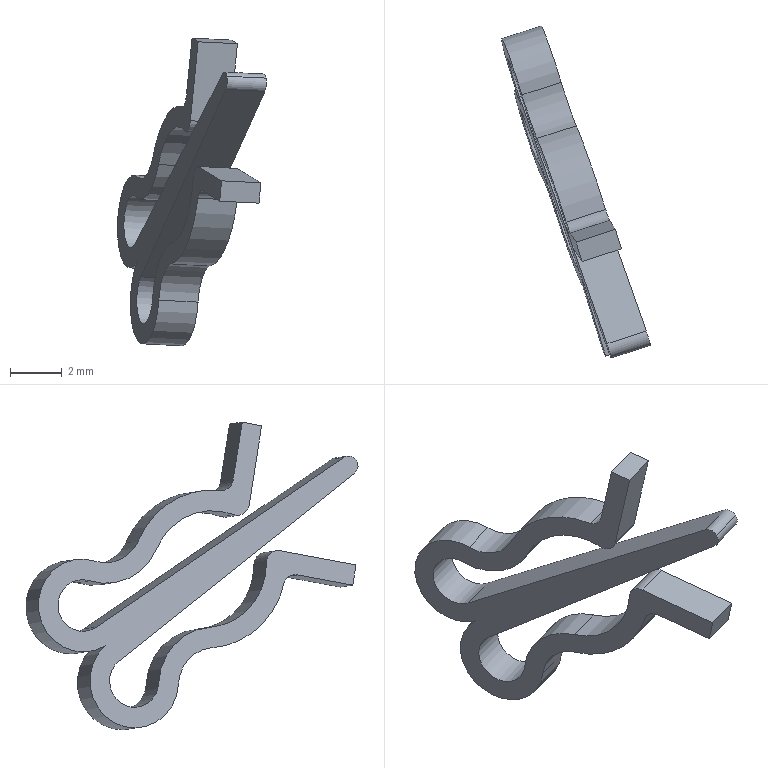Part | SolidWorks | features BaseBody 1 | 1 solid | 28 faces | box 5.768 x 12.862 x 11.907 mm | volume 63.823 mm3 | cylinder 18 | plane 10 | commonest cylinder face diameters 0.745 x2 0.982 x2 1 x2 2 x2 3 x2 3.6 x2
STEP:
#1=CARTESIAN_POINT('',(66.487,-82.448,-179.895));
#2=VERTEX_POINT('',#1);
#3=CARTESIAN_POINT('',(66.439,-82.377,-180.405));
#4=VERTEX_POINT('',#3);
#5=CARTESIAN_POINT('',(66.384,-82.16,-180.108));
#6=DIRECTION('',(0.9511,0.3055,-0.04654));
#7=DIRECTION('',(-0.2762,0.7728,-0.5713));
#8=AXIS2_PLACEMENT_3D('',#5,#6,#7);
#9=CIRCLE('',#8,0.3723);
#10=EDGE_CURVE('',#2,#4,#9,.T.);
#11=ORIENTED_EDGE('',*,*,#10,.F.);
#12=CARTESIAN_POINT('',(64.965,-82.936,-179.82));
#13=VERTEX_POINT('',#12);
#14=CARTESIAN_POINT('',(66.487,-82.448,-179.895));
#15=DIRECTION('',(-0.9511,-0.3055,0.04654));
#16=VECTOR('',#15,1000.);
#17=LINE('',#14,#16);
#18=EDGE_CURVE('',#2,#13,#17,.T.);
#19=ORIENTED_EDGE('',*,*,#18,.T.);
#20=CARTESIAN_POINT('',(64.918,-82.866,-180.331));
#21=VERTEX_POINT('',#20);
#22=CARTESIAN_POINT('',(64.863,-82.649,-180.033));
#23=DIRECTION('',(0.9511,0.3055,-0.04654));
#24=DIRECTION('',(-0.2762,0.7728,-0.5713));
#25=AXIS2_PLACEMENT_3D('',#22,#23,#24);
#26=CIRCLE('',#25,0.3723);
#27=EDGE_CURVE('',#13,#21,#26,.T.);
#28=ORIENTED_EDGE('',*,*,#27,.T.);
#29=CARTESIAN_POINT('',(66.439,-82.377,-180.405));
#30=DIRECTION('',(-0.9511,-0.3055,0.04654));
#31=VECTOR('',#30,1000.);
#32=LINE('',#29,#31);
#33=EDGE_CURVE('',#4,#21,#32,.T.);
#34=ORIENTED_EDGE('',*,*,#33,.F.);
#35=EDGE_LOOP('',(#11,#19,#28,#34));
#36=FACE_OUTER_BOUND('',#35,.T.);
#37=CARTESIAN_POINT('',(66.384,-82.16,-180.108));
#38=DIRECTION('',(-0.9511,-0.3055,0.04654));
#39=DIRECTION('',(0.2762,-0.7728,0.5713));
#40=AXIS2_PLACEMENT_3D('',#37,#38,#39);
#41=CYLINDRICAL_SURFACE('',#40,0.3723);
#42=ADVANCED_FACE('',(#36),#41,.T.);
#43=CARTESIAN_POINT('',(64.815,-82.452,-179.721));
#44=VERTEX_POINT('',#43);
#45=CARTESIAN_POINT('',(64.863,-82.649,-180.033));
#46=DIRECTION('',(0.9511,0.3055,-0.04654));
#47=DIRECTION('',(-0.2762,0.7728,-0.5713));
#48=AXIS2_PLACEMENT_3D('',#45,#46,#47);
#49=CIRCLE('',#48,0.3723);
#50=EDGE_CURVE('',#44,#13,#49,.T.);
#51=ORIENTED_EDGE('',*,*,#50,.F.);
#52=CARTESIAN_POINT('',(61.417,-72.873,-186.282));
#53=VERTEX_POINT('',#52);
#54=CARTESIAN_POINT('',(64.815,-82.452,-179.721));
#55=DIRECTION('',(0.2809,-0.7918,0.5424));
#56=VECTOR('',#55,1000.);
#57=LINE('',#54,#56);
#58=EDGE_CURVE('',#53,#44,#57,.T.);
#59=ORIENTED_EDGE('',*,*,#58,.F.);
#60=CARTESIAN_POINT('',(61.419,-72.607,-184.488));
#61=VERTEX_POINT('',#60);
#62=CARTESIAN_POINT('',(61.288,-72.344,-185.444));
#63=DIRECTION('',(-0.9511,-0.3055,0.04654));
#64=DIRECTION('',(-0.2762,0.7728,-0.5713));
#65=AXIS2_PLACEMENT_3D('',#62,#63,#64);
#66=CIRCLE('',#65,1.);
#67=EDGE_CURVE('',#61,#53,#66,.T.);
#68=ORIENTED_EDGE('',*,*,#67,.F.);
#69=CARTESIAN_POINT('',(62.319,-75.217,-183.241));
#70=VERTEX_POINT('',#69);
#71=CARTESIAN_POINT('',(61.721,-73.211,-182.289));
#72=DIRECTION('',(0.9511,0.3055,-0.04654));
#73=DIRECTION('',(-0.2762,0.7728,-0.5713));
#74=AXIS2_PLACEMENT_3D('',#71,#72,#73);
#75=CIRCLE('',#74,2.3);
#76=EDGE_CURVE('',#70,#61,#75,.T.);
#77=ORIENTED_EDGE('',*,*,#76,.F.);
#78=CARTESIAN_POINT('',(63.335,-78.182,-181.921));
#79=VERTEX_POINT('',#78);
#80=CARTESIAN_POINT('',(62.971,-77.406,-184.279));
#81=DIRECTION('',(-0.9511,-0.3055,0.04654));
#82=DIRECTION('',(-0.2762,0.7728,-0.5713));
#83=AXIS2_PLACEMENT_3D('',#80,#81,#82);
#84=CIRCLE('',#83,2.509);
#85=EDGE_CURVE('',#79,#70,#84,.T.);
#86=ORIENTED_EDGE('',*,*,#85,.F.);
#87=CARTESIAN_POINT('',(63.551,-78.795,-181.546));
#88=VERTEX_POINT('',#87);
#89=CARTESIAN_POINT('',(63.407,-78.334,-181.46));
#90=DIRECTION('',(0.9511,0.3055,-0.04654));
#91=DIRECTION('',(0.2762,-0.7728,0.5713));
#92=AXIS2_PLACEMENT_3D('',#89,#90,#91);
#93=CIRCLE('',#92,0.491);
#94=EDGE_CURVE('',#88,#79,#93,.T.);
#95=ORIENTED_EDGE('',*,*,#94,.F.);
#96=CARTESIAN_POINT('',(63.853,-79.272,-178.489));
#97=VERTEX_POINT('',#96);
#98=CARTESIAN_POINT('',(63.853,-79.272,-178.489));
#99=DIRECTION('',(-0.09732,0.1532,-0.9834));
#100=VECTOR('',#99,1000.);
#101=LINE('',#98,#100);
#102=EDGE_CURVE('',#97,#88,#101,.T.);
#103=ORIENTED_EDGE('',*,*,#102,.F.);
#104=CARTESIAN_POINT('',(63.619,-78.52,-178.348));
#105=VERTEX_POINT('',#104);
#106=CARTESIAN_POINT('',(63.853,-79.272,-178.489));
#107=DIRECTION('',(0.2933,-0.9398,-0.1754));
#108=VECTOR('',#107,1000.);
#109=LINE('',#106,#108);
#110=EDGE_CURVE('',#105,#97,#109,.T.);
#111=ORIENTED_EDGE('',*,*,#110,.F.);
#112=CARTESIAN_POINT('',(63.397,-78.171,-180.587));
#113=VERTEX_POINT('',#112);
#114=CARTESIAN_POINT('',(63.619,-78.52,-178.348));
#115=DIRECTION('',(0.09732,-0.1532,0.9834));
#116=VECTOR('',#115,1000.);
#117=LINE('',#114,#116);
#118=EDGE_CURVE('',#113,#105,#117,.T.);
#119=ORIENTED_EDGE('',*,*,#118,.F.);
#120=CARTESIAN_POINT('',(63.24,-77.743,-180.997));
#121=VERTEX_POINT('',#120);
#122=CARTESIAN_POINT('',(63.251,-77.701,-180.499));
#123=DIRECTION('',(-0.9511,-0.3055,0.04654));
#124=DIRECTION('',(-0.2762,0.7728,-0.5713));
#125=AXIS2_PLACEMENT_3D('',#122,#123,#124);
#126=CIRCLE('',#125,0.5);
#127=EDGE_CURVE('',#121,#113,#126,.T.);
#128=ORIENTED_EDGE('',*,*,#127,.F.);
#129=CARTESIAN_POINT('',(62.103,-74.502,-182.95));
#130=VERTEX_POINT('',#129);
#131=CARTESIAN_POINT('',(62.971,-77.406,-184.279));
#132=DIRECTION('',(0.9511,0.3055,-0.04654));
#133=DIRECTION('',(-0.2762,0.7728,-0.5713));
#134=AXIS2_PLACEMENT_3D('',#131,#132,#133);
#135=CIRCLE('',#134,3.31);
#136=EDGE_CURVE('',#130,#121,#135,.T.);
#137=ORIENTED_EDGE('',*,*,#136,.F.);
#138=CARTESIAN_POINT('',(61.524,-72.817,-183.723));
#139=VERTEX_POINT('',#138);
#140=CARTESIAN_POINT('',(61.721,-73.211,-182.289));
#141=DIRECTION('',(-0.9511,-0.3055,0.04654));
#142=DIRECTION('',(-0.2762,0.7728,-0.5713));
#143=AXIS2_PLACEMENT_3D('',#140,#141,#142);
#144=CIRCLE('',#143,1.5);
#145=EDGE_CURVE('',#139,#130,#144,.T.);
#146=ORIENTED_EDGE('',*,*,#145,.F.);
#147=CARTESIAN_POINT('',(61.495,-73.225,-187.));
#148=VERTEX_POINT('',#147);
#149=CARTESIAN_POINT('',(61.288,-72.344,-185.444));
#150=DIRECTION('',(0.9511,0.3055,-0.04654));
#151=DIRECTION('',(-0.2762,0.7728,-0.5713));
#152=AXIS2_PLACEMENT_3D('',#149,#150,#151);
#153=CIRCLE('',#152,1.8);
#154=EDGE_CURVE('',#148,#139,#153,.T.);
#155=ORIENTED_EDGE('',*,*,#154,.F.);
#156=CARTESIAN_POINT('',(62.33,-76.052,-188.489));
#157=VERTEX_POINT('',#156);
#158=CARTESIAN_POINT('',(61.785,-74.339,-188.383));
#159=DIRECTION('',(0.9511,0.3055,-0.04654));
#160=DIRECTION('',(0.2762,-0.7728,0.5713));
#161=AXIS2_PLACEMENT_3D('',#158,#159,#160);
#162=CIRCLE('',#161,1.8);
#163=EDGE_CURVE('',#157,#148,#162,.T.);
#164=ORIENTED_EDGE('',*,*,#163,.F.);
#165=CARTESIAN_POINT('',(62.802,-77.309,-187.086));
#166=VERTEX_POINT('',#165);
#167=CARTESIAN_POINT('',(62.784,-77.479,-188.576));
#168=DIRECTION('',(-0.9511,-0.3055,0.04654));
#169=DIRECTION('',(0.2762,-0.7728,0.5713));
#170=AXIS2_PLACEMENT_3D('',#167,#168,#169);
#171=CIRCLE('',#170,1.5);
#172=EDGE_CURVE('',#166,#157,#171,.T.);
#173=ORIENTED_EDGE('',*,*,#172,.F.);
#174=CARTESIAN_POINT('',(63.839,-80.15,-184.543));
#175=VERTEX_POINT('',#174);
#176=CARTESIAN_POINT('',(62.887,-77.071,-183.786));
#177=DIRECTION('',(0.9511,0.3055,-0.04654));
#178=DIRECTION('',(0.2762,-0.7728,0.5713));
#179=AXIS2_PLACEMENT_3D('',#176,#177,#178);
#180=CIRCLE('',#179,3.31);
#181=EDGE_CURVE('',#175,#166,#180,.T.);
#182=ORIENTED_EDGE('',*,*,#181,.F.);
#183=CARTESIAN_POINT('',(64.018,-80.663,-184.258));
#184=VERTEX_POINT('',#183);
#185=CARTESIAN_POINT('',(63.969,-80.586,-184.749));
#186=DIRECTION('',(-0.9511,-0.3055,0.04654));
#187=DIRECTION('',(0.2762,-0.7728,0.5713));
#188=AXIS2_PLACEMENT_3D('',#185,#186,#187);
#189=CIRCLE('',#188,0.5);
#190=EDGE_CURVE('',#184,#175,#189,.T.);
#191=ORIENTED_EDGE('',*,*,#190,.F.);
#192=CARTESIAN_POINT('',(64.686,-82.802,-184.657));
#193=VERTEX_POINT('',#192);
#194=CARTESIAN_POINT('',(64.686,-82.802,-184.657));
#195=DIRECTION('',(-0.2933,0.9398,0.1754));
#196=VECTOR('',#195,1000.);
#197=LINE('',#194,#196);
#198=EDGE_CURVE('',#193,#184,#197,.T.);
#199=ORIENTED_EDGE('',*,*,#198,.F.);
#200=CARTESIAN_POINT('',(64.763,-82.925,-183.87));
#201=VERTEX_POINT('',#200);
#202=CARTESIAN_POINT('',(64.763,-82.925,-183.87));
#203=DIRECTION('',(-0.09732,0.1532,-0.9834));
#204=VECTOR('',#203,1000.);
#205=LINE('',#202,#204);
#206=EDGE_CURVE('',#201,#193,#205,.T.);
#207=ORIENTED_EDGE('',*,*,#206,.F.);
#208=CARTESIAN_POINT('',(63.852,-80.003,-183.325));
#209=VERTEX_POINT('',#208);
#210=CARTESIAN_POINT('',(64.763,-82.925,-183.87));
#211=DIRECTION('',(0.2933,-0.9398,-0.1754));
#212=VECTOR('',#211,1000.);
#213=LINE('',#210,#212);
#214=EDGE_CURVE('',#209,#201,#213,.T.);
#215=ORIENTED_EDGE('',*,*,#214,.F.);
#216=CARTESIAN_POINT('',(63.654,-79.46,-183.804));
#217=VERTEX_POINT('',#216);
#218=CARTESIAN_POINT('',(63.804,-79.928,-183.808));
#219=DIRECTION('',(0.9511,0.3055,-0.04654));
#220=DIRECTION('',(-0.2762,0.7728,-0.5713));
#221=AXIS2_PLACEMENT_3D('',#218,#219,#220);
#222=CIRCLE('',#221,0.491);
#223=EDGE_CURVE('',#217,#209,#222,.T.);
#224=ORIENTED_EDGE('',*,*,#223,.F.);
#225=CARTESIAN_POINT('',(62.833,-77.284,-186.285));
#226=VERTEX_POINT('',#225);
#227=CARTESIAN_POINT('',(62.887,-77.071,-183.786));
#228=DIRECTION('',(-0.9511,-0.3055,0.04654));
#229=DIRECTION('',(0.2762,-0.7728,0.5713));
#230=AXIS2_PLACEMENT_3D('',#227,#228,#229);
#231=CIRCLE('',#230,2.509);
#232=EDGE_CURVE('',#226,#217,#231,.T.);
#233=ORIENTED_EDGE('',*,*,#232,.F.);
#234=CARTESIAN_POINT('',(62.088,-75.291,-188.442));
#235=VERTEX_POINT('',#234);
#236=CARTESIAN_POINT('',(62.784,-77.479,-188.576));
#237=DIRECTION('',(0.9511,0.3055,-0.04654));
#238=DIRECTION('',(0.2762,-0.7728,0.5713));
#239=AXIS2_PLACEMENT_3D('',#236,#237,#238);
#240=CIRCLE('',#239,2.3);
#241=EDGE_CURVE('',#235,#226,#240,.T.);
#242=ORIENTED_EDGE('',*,*,#241,.F.);
#243=CARTESIAN_POINT('',(61.637,-73.757,-187.584));
#244=VERTEX_POINT('',#243);
#245=CARTESIAN_POINT('',(61.785,-74.339,-188.383));
#246=DIRECTION('',(-0.9511,-0.3055,0.04654));
#247=DIRECTION('',(0.2762,-0.7728,0.5713));
#248=AXIS2_PLACEMENT_3D('',#245,#246,#247);
#249=CIRCLE('',#248,1.);
#250=EDGE_CURVE('',#244,#235,#249,.T.);
#251=ORIENTED_EDGE('',*,*,#250,.F.);
#252=CARTESIAN_POINT('',(64.918,-82.866,-180.331));
#253=DIRECTION('',(-0.2712,0.753,-0.5996));
#254=VECTOR('',#253,1000.);
#255=LINE('',#252,#254);
#256=EDGE_CURVE('',#21,#244,#255,.T.);
#257=ORIENTED_EDGE('',*,*,#256,.F.);
#258=ORIENTED_EDGE('',*,*,#27,.F.);
#259=EDGE_LOOP('',(#51,#59,#68,#77,#86,#95,#103,#111,#119,#128,#137,#146,#155,#164,#173,#182,#191,#199,#207,#215,#224,#233,#242,#251,#257,#258));
#260=FACE_OUTER_BOUND('',#259,.T.);
#261=CARTESIAN_POINT('',(64.863,-82.649,-180.033));
#262=DIRECTION('',(0.9511,0.3055,-0.04654));
#263=DIRECTION('',(0.,-0.1506,-0.9886));
#264=AXIS2_PLACEMENT_3D('',#261,#262,#263);
#265=PLANE('',#264);
#266=ADVANCED_FACE('',(#260),#265,.F.);
#267=CARTESIAN_POINT('',(66.336,-81.963,-179.795));
#268=VERTEX_POINT('',#267);
#269=CARTESIAN_POINT('',(66.384,-82.16,-180.108));
#270=DIRECTION('',(0.9511,0.3055,-0.04654));
#271=DIRECTION('',(-0.2762,0.7728,-0.5713));
#272=AXIS2_PLACEMENT_3D('',#269,#270,#271);
#273=CIRCLE('',#272,0.3723);
#274=EDGE_CURVE('',#268,#2,#273,.T.);
#275=ORIENTED_EDGE('',*,*,#274,.T.);
#276=ORIENTED_EDGE('',*,*,#10,.T.);
#277=CARTESIAN_POINT('',(63.158,-73.268,-187.659));
#278=VERTEX_POINT('',#277);
#279=CARTESIAN_POINT('',(66.439,-82.377,-180.405));
#280=DIRECTION('',(-0.2712,0.753,-0.5996));
#281=VECTOR('',#280,1000.);
#282=LINE('',#279,#281);
#283=EDGE_CURVE('',#4,#278,#282,.T.);
#284=ORIENTED_EDGE('',*,*,#283,.T.);
#285=CARTESIAN_POINT('',(63.609,-74.802,-188.516));
#286=VERTEX_POINT('',#285);
#287=CARTESIAN_POINT('',(63.307,-73.851,-188.458));
#288=DIRECTION('',(-0.9511,-0.3055,0.04654));
#289=DIRECTION('',(0.2762,-0.7728,0.5713));
#290=AXIS2_PLACEMENT_3D('',#287,#288,#289);
#291=CIRCLE('',#290,1.);
#292=EDGE_CURVE('',#278,#286,#291,.T.);
#293=ORIENTED_EDGE('',*,*,#292,.T.);
#294=CARTESIAN_POINT('',(64.355,-76.795,-186.36));
#295=VERTEX_POINT('',#294);
#296=CARTESIAN_POINT('',(64.306,-76.99,-188.651));
#297=DIRECTION('',(0.9511,0.3055,-0.04654));
#298=DIRECTION('',(0.2762,-0.7728,0.5713));
#299=AXIS2_PLACEMENT_3D('',#296,#297,#298);
#300=CIRCLE('',#299,2.3);
#301=EDGE_CURVE('',#286,#295,#300,.T.);
#302=ORIENTED_EDGE('',*,*,#301,.T.);
#303=CARTESIAN_POINT('',(65.176,-78.971,-183.879));
#304=VERTEX_POINT('',#303);
#305=CARTESIAN_POINT('',(64.409,-76.583,-183.86));
#306=DIRECTION('',(-0.9511,-0.3055,0.04654));
#307=DIRECTION('',(0.2762,-0.7728,0.5713));
#308=AXIS2_PLACEMENT_3D('',#305,#306,#307);
#309=CIRCLE('',#308,2.509);
#310=EDGE_CURVE('',#295,#304,#309,.T.);
#311=ORIENTED_EDGE('',*,*,#310,.T.);
#312=CARTESIAN_POINT('',(65.373,-79.514,-183.399));
#313=VERTEX_POINT('',#312);
#314=CARTESIAN_POINT('',(65.326,-79.439,-183.882));
#315=DIRECTION('',(0.9511,0.3055,-0.04654));
#316=DIRECTION('',(-0.2762,0.7728,-0.5713));
#317=AXIS2_PLACEMENT_3D('',#314,#315,#316);
#318=CIRCLE('',#317,0.491);
#319=EDGE_CURVE('',#304,#313,#318,.T.);
#320=ORIENTED_EDGE('',*,*,#319,.T.);
#321=CARTESIAN_POINT('',(66.285,-82.436,-183.945));
#322=VERTEX_POINT('',#321);
#323=CARTESIAN_POINT('',(66.285,-82.436,-183.945));
#324=DIRECTION('',(0.2933,-0.9398,-0.1754));
#325=VECTOR('',#324,1000.);
#326=LINE('',#323,#325);
#327=EDGE_CURVE('',#313,#322,#326,.T.);
#328=ORIENTED_EDGE('',*,*,#327,.T.);
#329=CARTESIAN_POINT('',(66.207,-82.313,-184.731));
#330=VERTEX_POINT('',#329);
#331=CARTESIAN_POINT('',(66.285,-82.436,-183.945));
#332=DIRECTION('',(-0.09732,0.1532,-0.9834));
#333=VECTOR('',#332,1000.);
#334=LINE('',#331,#333);
#335=EDGE_CURVE('',#322,#330,#334,.T.);
#336=ORIENTED_EDGE('',*,*,#335,.T.);
#337=CARTESIAN_POINT('',(65.54,-80.174,-184.332));
#338=VERTEX_POINT('',#337);
#339=CARTESIAN_POINT('',(66.207,-82.313,-184.731));
#340=DIRECTION('',(-0.2933,0.9398,0.1754));
#341=VECTOR('',#340,1000.);
#342=LINE('',#339,#341);
#343=EDGE_CURVE('',#330,#338,#342,.T.);
#344=ORIENTED_EDGE('',*,*,#343,.T.);
#345=CARTESIAN_POINT('',(65.361,-79.661,-184.617));
#346=VERTEX_POINT('',#345);
#347=CARTESIAN_POINT('',(65.491,-80.097,-184.824));
#348=DIRECTION('',(-0.9511,-0.3055,0.04654));
#349=DIRECTION('',(0.2762,-0.7728,0.5713));
#350=AXIS2_PLACEMENT_3D('',#347,#348,#349);
#351=CIRCLE('',#350,0.5);
#352=EDGE_CURVE('',#338,#346,#351,.T.);
#353=ORIENTED_EDGE('',*,*,#352,.T.);
#354=CARTESIAN_POINT('',(64.324,-76.82,-187.161));
#355=VERTEX_POINT('',#354);
#356=CARTESIAN_POINT('',(64.409,-76.583,-183.86));
#357=DIRECTION('',(0.9511,0.3055,-0.04654));
#358=DIRECTION('',(0.2762,-0.7728,0.5713));
#359=AXIS2_PLACEMENT_3D('',#356,#357,#358);
#360=CIRCLE('',#359,3.31);
#361=EDGE_CURVE('',#346,#355,#360,.T.);
#362=ORIENTED_EDGE('',*,*,#361,.T.);
#363=CARTESIAN_POINT('',(63.851,-75.563,-188.563));
#364=VERTEX_POINT('',#363);
#365=CARTESIAN_POINT('',(64.306,-76.99,-188.651));
#366=DIRECTION('',(-0.9511,-0.3055,0.04654));
#367=DIRECTION('',(0.2762,-0.7728,0.5713));
#368=AXIS2_PLACEMENT_3D('',#365,#366,#367);
#369=CIRCLE('',#368,1.5);
#370=EDGE_CURVE('',#355,#364,#369,.T.);
#371=ORIENTED_EDGE('',*,*,#370,.T.);
#372=CARTESIAN_POINT('',(63.016,-72.736,-187.074));
#373=VERTEX_POINT('',#372);
#374=CARTESIAN_POINT('',(63.307,-73.851,-188.458));
#375=DIRECTION('',(0.9511,0.3055,-0.04654));
#376=DIRECTION('',(0.2762,-0.7728,0.5713));
#377=AXIS2_PLACEMENT_3D('',#374,#375,#376);
#378=CIRCLE('',#377,1.8);
#379=EDGE_CURVE('',#364,#373,#378,.T.);
#380=ORIENTED_EDGE('',*,*,#379,.T.);
#381=CARTESIAN_POINT('',(63.046,-72.328,-183.797));
#382=VERTEX_POINT('',#381);
#383=CARTESIAN_POINT('',(62.81,-71.855,-185.518));
#384=DIRECTION('',(0.9511,0.3055,-0.04654));
#385=DIRECTION('',(-0.2762,0.7728,-0.5713));
#386=AXIS2_PLACEMENT_3D('',#383,#384,#385);
#387=CIRCLE('',#386,1.8);
#388=EDGE_CURVE('',#373,#382,#387,.T.);
#389=ORIENTED_EDGE('',*,*,#388,.T.);
#390=CARTESIAN_POINT('',(63.625,-74.013,-183.025));
#391=VERTEX_POINT('',#390);
#392=CARTESIAN_POINT('',(63.242,-72.722,-182.363));
#393=DIRECTION('',(-0.9511,-0.3055,0.04654));
#394=DIRECTION('',(-0.2762,0.7728,-0.5713));
#395=AXIS2_PLACEMENT_3D('',#392,#393,#394);
#396=CIRCLE('',#395,1.5);
#397=EDGE_CURVE('',#382,#391,#396,.T.);
#398=ORIENTED_EDGE('',*,*,#397,.T.);
#399=CARTESIAN_POINT('',(64.761,-77.254,-181.072));
#400=VERTEX_POINT('',#399);
#401=CARTESIAN_POINT('',(64.492,-76.917,-184.354));
#402=DIRECTION('',(0.9511,0.3055,-0.04654));
#403=DIRECTION('',(-0.2762,0.7728,-0.5713));
#404=AXIS2_PLACEMENT_3D('',#401,#402,#403);
#405=CIRCLE('',#404,3.31);
#406=EDGE_CURVE('',#391,#400,#405,.T.);
#407=ORIENTED_EDGE('',*,*,#406,.T.);
#408=CARTESIAN_POINT('',(64.919,-77.682,-180.661));
#409=VERTEX_POINT('',#408);
#410=CARTESIAN_POINT('',(64.772,-77.212,-180.574));
#411=DIRECTION('',(-0.9511,-0.3055,0.04654));
#412=DIRECTION('',(-0.2762,0.7728,-0.5713));
#413=AXIS2_PLACEMENT_3D('',#410,#411,#412);
#414=CIRCLE('',#413,0.5);
#415=EDGE_CURVE('',#400,#409,#414,.T.);
#416=ORIENTED_EDGE('',*,*,#415,.T.);
#417=CARTESIAN_POINT('',(65.14,-78.031,-178.423));
#418=VERTEX_POINT('',#417);
#419=CARTESIAN_POINT('',(65.14,-78.031,-178.423));
#420=DIRECTION('',(0.09732,-0.1532,0.9834));
#421=VECTOR('',#420,1000.);
#422=LINE('',#419,#421);
#423=EDGE_CURVE('',#409,#418,#422,.T.);
#424=ORIENTED_EDGE('',*,*,#423,.T.);
#425=CARTESIAN_POINT('',(65.375,-78.783,-178.563));
#426=VERTEX_POINT('',#425);
#427=CARTESIAN_POINT('',(65.375,-78.783,-178.563));
#428=DIRECTION('',(0.2933,-0.9398,-0.1754));
#429=VECTOR('',#428,1000.);
#430=LINE('',#427,#429);
#431=EDGE_CURVE('',#418,#426,#430,.T.);
#432=ORIENTED_EDGE('',*,*,#431,.T.);
#433=CARTESIAN_POINT('',(65.072,-78.307,-181.62));
#434=VERTEX_POINT('',#433);
#435=CARTESIAN_POINT('',(65.375,-78.783,-178.563));
#436=DIRECTION('',(-0.09732,0.1532,-0.9834));
#437=VECTOR('',#436,1000.);
#438=LINE('',#435,#437);
#439=EDGE_CURVE('',#426,#434,#438,.T.);
#440=ORIENTED_EDGE('',*,*,#439,.T.);
#441=CARTESIAN_POINT('',(64.857,-77.693,-181.996));
#442=VERTEX_POINT('',#441);
#443=CARTESIAN_POINT('',(64.928,-77.845,-181.534));
#444=DIRECTION('',(0.9511,0.3055,-0.04654));
#445=DIRECTION('',(0.2762,-0.7728,0.5713));
#446=AXIS2_PLACEMENT_3D('',#443,#444,#445);
#447=CIRCLE('',#446,0.491);
#448=EDGE_CURVE('',#434,#442,#447,.T.);
#449=ORIENTED_EDGE('',*,*,#448,.T.);
#450=CARTESIAN_POINT('',(63.84,-74.728,-183.315));
#451=VERTEX_POINT('',#450);
#452=CARTESIAN_POINT('',(64.492,-76.917,-184.354));
#453=DIRECTION('',(-0.9511,-0.3055,0.04654));
#454=DIRECTION('',(-0.2762,0.7728,-0.5713));
#455=AXIS2_PLACEMENT_3D('',#452,#453,#454);
#456=CIRCLE('',#455,2.509);
#457=EDGE_CURVE('',#442,#451,#456,.T.);
#458=ORIENTED_EDGE('',*,*,#457,.T.);
#459=CARTESIAN_POINT('',(62.941,-72.118,-184.562));
#460=VERTEX_POINT('',#459);
#461=CARTESIAN_POINT('',(63.242,-72.722,-182.363));
#462=DIRECTION('',(0.9511,0.3055,-0.04654));
#463=DIRECTION('',(-0.2762,0.7728,-0.5713));
#464=AXIS2_PLACEMENT_3D('',#461,#462,#463);
#465=CIRCLE('',#464,2.3);
#466=EDGE_CURVE('',#451,#460,#465,.T.);
#467=ORIENTED_EDGE('',*,*,#466,.T.);
#468=CARTESIAN_POINT('',(62.938,-72.384,-186.357));
#469=VERTEX_POINT('',#468);
#470=CARTESIAN_POINT('',(62.81,-71.855,-185.518));
#471=DIRECTION('',(-0.9511,-0.3055,0.04654));
#472=DIRECTION('',(-0.2762,0.7728,-0.5713));
#473=AXIS2_PLACEMENT_3D('',#470,#471,#472);
#474=CIRCLE('',#473,1.);
#475=EDGE_CURVE('',#460,#469,#474,.T.);
#476=ORIENTED_EDGE('',*,*,#475,.T.);
#477=CARTESIAN_POINT('',(66.336,-81.963,-179.795));
#478=DIRECTION('',(0.2809,-0.7918,0.5424));
#479=VECTOR('',#478,1000.);
#480=LINE('',#477,#479);
#481=EDGE_CURVE('',#469,#268,#480,.T.);
#482=ORIENTED_EDGE('',*,*,#481,.T.);
#483=EDGE_LOOP('',(#275,#276,#284,#293,#302,#311,#320,#328,#336,#344,#353,#362,#371,#380,#389,#398,#407,#416,#424,#432,#440,#449,#458,#467,#476,#482));
#484=FACE_OUTER_BOUND('',#483,.T.);
#485=CARTESIAN_POINT('',(66.384,-82.16,-180.108));
#486=DIRECTION('',(0.9511,0.3055,-0.04654));
#487=DIRECTION('',(0.,-0.1506,-0.9886));
#488=AXIS2_PLACEMENT_3D('',#485,#486,#487);
#489=PLANE('',#488);
#490=ADVANCED_FACE('',(#484),#489,.T.);
#491=ORIENTED_EDGE('',*,*,#58,.T.);
#492=CARTESIAN_POINT('',(66.336,-81.963,-179.795));
#493=DIRECTION('',(-0.9511,-0.3055,0.04654));
#494=VECTOR('',#493,1000.);
#495=LINE('',#492,#494);
#496=EDGE_CURVE('',#268,#44,#495,.T.);
#497=ORIENTED_EDGE('',*,*,#496,.F.);
#498=ORIENTED_EDGE('',*,*,#481,.F.);
#499=CARTESIAN_POINT('',(62.938,-72.384,-186.357));
#500=DIRECTION('',(-0.9511,-0.3055,0.04654));
#501=VECTOR('',#500,1000.);
#502=LINE('',#499,#501);
#503=EDGE_CURVE('',#469,#53,#502,.T.);
#504=ORIENTED_EDGE('',*,*,#503,.T.);
#505=EDGE_LOOP('',(#491,#497,#498,#504));
#506=FACE_OUTER_BOUND('',#505,.T.);
#507=CARTESIAN_POINT('',(66.336,-81.963,-179.795));
#508=DIRECTION('',(0.1288,-0.5289,-0.8388));
#509=DIRECTION('',(0.,-0.8459,0.5334));
#510=AXIS2_PLACEMENT_3D('',#507,#508,#509);
#511=PLANE('',#510);
#512=ADVANCED_FACE('',(#506),#511,.F.);
#513=ORIENTED_EDGE('',*,*,#67,.T.);
#514=ORIENTED_EDGE('',*,*,#503,.F.);
#515=ORIENTED_EDGE('',*,*,#475,.F.);
#516=CARTESIAN_POINT('',(62.941,-72.118,-184.562));
#517=DIRECTION('',(-0.9511,-0.3055,0.04654));
#518=VECTOR('',#517,1000.);
#519=LINE('',#516,#518);
#520=EDGE_CURVE('',#460,#61,#519,.T.);
#521=ORIENTED_EDGE('',*,*,#520,.T.);
#522=EDGE_LOOP('',(#513,#514,#515,#521));
#523=FACE_OUTER_BOUND('',#522,.T.);
#524=CARTESIAN_POINT('',(62.81,-71.855,-185.518));
#525=DIRECTION('',(-0.9511,-0.3055,0.04654));
#526=DIRECTION('',(0.2762,-0.7728,0.5713));
#527=AXIS2_PLACEMENT_3D('',#524,#525,#526);
#528=CYLINDRICAL_SURFACE('',#527,1.);
#529=ADVANCED_FACE('',(#523),#528,.F.);
#530=ORIENTED_EDGE('',*,*,#76,.T.);
#531=ORIENTED_EDGE('',*,*,#520,.F.);
#532=ORIENTED_EDGE('',*,*,#466,.F.);
#533=CARTESIAN_POINT('',(63.84,-74.728,-183.315));
#534=DIRECTION('',(-0.9511,-0.3055,0.04654));
#535=VECTOR('',#534,1000.);
#536=LINE('',#533,#535);
#537=EDGE_CURVE('',#451,#70,#536,.T.);
#538=ORIENTED_EDGE('',*,*,#537,.T.);
#539=EDGE_LOOP('',(#530,#531,#532,#538));
#540=FACE_OUTER_BOUND('',#539,.T.);
#541=CARTESIAN_POINT('',(63.242,-72.722,-182.363));
#542=DIRECTION('',(-0.9511,-0.3055,0.04654));
#543=DIRECTION('',(0.2762,-0.7728,0.5713));
#544=AXIS2_PLACEMENT_3D('',#541,#542,#543);
#545=CYLINDRICAL_SURFACE('',#544,2.3);
#546=ADVANCED_FACE('',(#540),#545,.T.);
#547=ORIENTED_EDGE('',*,*,#85,.T.);
#548=ORIENTED_EDGE('',*,*,#537,.F.);
#549=ORIENTED_EDGE('',*,*,#457,.F.);
#550=CARTESIAN_POINT('',(64.857,-77.693,-181.996));
#551=DIRECTION('',(-0.9511,-0.3055,0.04654));
#552=VECTOR('',#551,1000.);
#553=LINE('',#550,#552);
#554=EDGE_CURVE('',#442,#79,#553,.T.);
#555=ORIENTED_EDGE('',*,*,#554,.T.);
#556=EDGE_LOOP('',(#547,#548,#549,#555));
#557=FACE_OUTER_BOUND('',#556,.T.);
#558=CARTESIAN_POINT('',(64.492,-76.917,-184.354));
#559=DIRECTION('',(-0.9511,-0.3055,0.04654));
#560=DIRECTION('',(0.2762,-0.7728,0.5713));
#561=AXIS2_PLACEMENT_3D('',#558,#559,#560);
#562=CYLINDRICAL_SURFACE('',#561,2.509);
#563=ADVANCED_FACE('',(#557),#562,.F.);
#564=ORIENTED_EDGE('',*,*,#94,.T.);
#565=ORIENTED_EDGE('',*,*,#554,.F.);
#566=ORIENTED_EDGE('',*,*,#448,.F.);
#567=CARTESIAN_POINT('',(65.072,-78.307,-181.62));
#568=DIRECTION('',(-0.9511,-0.3055,0.04654));
#569=VECTOR('',#568,1000.);
#570=LINE('',#567,#569);
#571=EDGE_CURVE('',#434,#88,#570,.T.);
#572=ORIENTED_EDGE('',*,*,#571,.T.);
#573=EDGE_LOOP('',(#564,#565,#566,#572));
#574=FACE_OUTER_BOUND('',#573,.T.);
#575=CARTESIAN_POINT('',(64.928,-77.845,-181.534));
#576=DIRECTION('',(-0.9511,-0.3055,0.04654));
#577=DIRECTION('',(0.2762,-0.7728,0.5713));
#578=AXIS2_PLACEMENT_3D('',#575,#576,#577);
#579=CYLINDRICAL_SURFACE('',#578,0.491);
#580=ADVANCED_FACE('',(#574),#579,.T.);
#581=ORIENTED_EDGE('',*,*,#102,.T.);
#582=ORIENTED_EDGE('',*,*,#571,.F.);
#583=ORIENTED_EDGE('',*,*,#439,.F.);
#584=CARTESIAN_POINT('',(65.375,-78.783,-178.563));
#585=DIRECTION('',(-0.9511,-0.3055,0.04654));
#586=VECTOR('',#585,1000.);
#587=LINE('',#584,#586);
#588=EDGE_CURVE('',#426,#97,#587,.T.);
#589=ORIENTED_EDGE('',*,*,#588,.T.);
#590=EDGE_LOOP('',(#581,#582,#583,#589));
#591=FACE_OUTER_BOUND('',#590,.T.);
#592=CARTESIAN_POINT('',(65.375,-78.783,-178.563));
#593=DIRECTION('',(-0.2933,0.9398,0.1754));
#594=DIRECTION('',(0.5133,0.,0.8582));
#595=AXIS2_PLACEMENT_3D('',#592,#593,#594);
#596=PLANE('',#595);
#597=ADVANCED_FACE('',(#591),#596,.F.);
#598=ORIENTED_EDGE('',*,*,#110,.T.);
#599=ORIENTED_EDGE('',*,*,#588,.F.);
#600=ORIENTED_EDGE('',*,*,#431,.F.);
#601=CARTESIAN_POINT('',(65.14,-78.031,-178.423));
#602=DIRECTION('',(-0.9511,-0.3055,0.04654));
#603=VECTOR('',#602,1000.);
#604=LINE('',#601,#603);
#605=EDGE_CURVE('',#418,#105,#604,.T.);
#606=ORIENTED_EDGE('',*,*,#605,.T.);
#607=EDGE_LOOP('',(#598,#599,#600,#606));
#608=FACE_OUTER_BOUND('',#607,.T.);
#609=CARTESIAN_POINT('',(65.375,-78.783,-178.563));
#610=DIRECTION('',(-0.09732,0.1532,-0.9834));
#611=DIRECTION('',(-0.9951,0.,0.09849));
#612=AXIS2_PLACEMENT_3D('',#609,#610,#611);
#613=PLANE('',#612);
#614=ADVANCED_FACE('',(#608),#613,.F.);
#615=ORIENTED_EDGE('',*,*,#118,.T.);
#616=ORIENTED_EDGE('',*,*,#605,.F.);
#617=ORIENTED_EDGE('',*,*,#423,.F.);
#618=CARTESIAN_POINT('',(64.919,-77.682,-180.661));
#619=DIRECTION('',(-0.9511,-0.3055,0.04654));
#620=VECTOR('',#619,1000.);
#621=LINE('',#618,#620);
#622=EDGE_CURVE('',#409,#113,#621,.T.);
#623=ORIENTED_EDGE('',*,*,#622,.T.);
#624=EDGE_LOOP('',(#615,#616,#617,#623));
#625=FACE_OUTER_BOUND('',#624,.T.);
#626=CARTESIAN_POINT('',(65.14,-78.031,-178.423));
#627=DIRECTION('',(0.2933,-0.9398,-0.1754));
#628=DIRECTION('',(0.,0.1835,-0.983));
#629=AXIS2_PLACEMENT_3D('',#626,#627,#628);
#630=PLANE('',#629);
#631=ADVANCED_FACE('',(#625),#630,.F.);
#632=ORIENTED_EDGE('',*,*,#127,.T.);
#633=ORIENTED_EDGE('',*,*,#622,.F.);
#634=ORIENTED_EDGE('',*,*,#415,.F.);
#635=CARTESIAN_POINT('',(64.761,-77.254,-181.072));
#636=DIRECTION('',(-0.9511,-0.3055,0.04654));
#637=VECTOR('',#636,1000.);
#638=LINE('',#635,#637);
#639=EDGE_CURVE('',#400,#121,#638,.T.);
#640=ORIENTED_EDGE('',*,*,#639,.T.);
#641=EDGE_LOOP('',(#632,#633,#634,#640));
#642=FACE_OUTER_BOUND('',#641,.T.);
#643=CARTESIAN_POINT('',(64.772,-77.212,-180.574));
#644=DIRECTION('',(-0.9511,-0.3055,0.04654));
#645=DIRECTION('',(0.2762,-0.7728,0.5713));
#646=AXIS2_PLACEMENT_3D('',#643,#644,#645);
#647=CYLINDRICAL_SURFACE('',#646,0.5);
#648=ADVANCED_FACE('',(#642),#647,.F.);
#649=ORIENTED_EDGE('',*,*,#136,.T.);
#650=ORIENTED_EDGE('',*,*,#639,.F.);
#651=ORIENTED_EDGE('',*,*,#406,.F.);
#652=CARTESIAN_POINT('',(63.625,-74.013,-183.025));
#653=DIRECTION('',(-0.9511,-0.3055,0.04654));
#654=VECTOR('',#653,1000.);
#655=LINE('',#652,#654);
#656=EDGE_CURVE('',#391,#130,#655,.T.);
#657=ORIENTED_EDGE('',*,*,#656,.T.);
#658=EDGE_LOOP('',(#649,#650,#651,#657));
#659=FACE_OUTER_BOUND('',#658,.T.);
#660=CARTESIAN_POINT('',(64.492,-76.917,-184.354));
#661=DIRECTION('',(-0.9511,-0.3055,0.04654));
#662=DIRECTION('',(0.2762,-0.7728,0.5713));
#663=AXIS2_PLACEMENT_3D('',#660,#661,#662);
#664=CYLINDRICAL_SURFACE('',#663,3.31);
#665=ADVANCED_FACE('',(#659),#664,.T.);
#666=ORIENTED_EDGE('',*,*,#145,.T.);
#667=ORIENTED_EDGE('',*,*,#656,.F.);
#668=ORIENTED_EDGE('',*,*,#397,.F.);
#669=CARTESIAN_POINT('',(63.046,-72.328,-183.797));
#670=DIRECTION('',(-0.9511,-0.3055,0.04654));
#671=VECTOR('',#670,1000.);
#672=LINE('',#669,#671);
#673=EDGE_CURVE('',#382,#139,#672,.T.);
#674=ORIENTED_EDGE('',*,*,#673,.T.);
#675=EDGE_LOOP('',(#666,#667,#668,#674));
#676=FACE_OUTER_BOUND('',#675,.T.);
#677=CARTESIAN_POINT('',(63.242,-72.722,-182.363));
#678=DIRECTION('',(-0.9511,-0.3055,0.04654));
#679=DIRECTION('',(0.2762,-0.7728,0.5713));
#680=AXIS2_PLACEMENT_3D('',#677,#678,#679);
#681=CYLINDRICAL_SURFACE('',#680,1.5);
#682=ADVANCED_FACE('',(#676),#681,.F.);
#683=ORIENTED_EDGE('',*,*,#154,.T.);
#684=ORIENTED_EDGE('',*,*,#673,.F.);
#685=ORIENTED_EDGE('',*,*,#388,.F.);
#686=CARTESIAN_POINT('',(63.016,-72.736,-187.074));
#687=DIRECTION('',(-0.9511,-0.3055,0.04654));
#688=VECTOR('',#687,1000.);
#689=LINE('',#686,#688);
#690=EDGE_CURVE('',#373,#148,#689,.T.);
#691=ORIENTED_EDGE('',*,*,#690,.T.);
#692=EDGE_LOOP('',(#683,#684,#685,#691));
#693=FACE_OUTER_BOUND('',#692,.T.);
#694=CARTESIAN_POINT('',(62.81,-71.855,-185.518));
#695=DIRECTION('',(-0.9511,-0.3055,0.04654));
#696=DIRECTION('',(0.2762,-0.7728,0.5713));
#697=AXIS2_PLACEMENT_3D('',#694,#695,#696);
#698=CYLINDRICAL_SURFACE('',#697,1.8);
#699=ADVANCED_FACE('',(#693),#698,.T.);
#700=ORIENTED_EDGE('',*,*,#163,.T.);
#701=ORIENTED_EDGE('',*,*,#690,.F.);
#702=ORIENTED_EDGE('',*,*,#379,.F.);
#703=CARTESIAN_POINT('',(63.851,-75.563,-188.563));
#704=DIRECTION('',(-0.9511,-0.3055,0.04654));
#705=VECTOR('',#704,1000.);
#706=LINE('',#703,#705);
#707=EDGE_CURVE('',#364,#157,#706,.T.);
#708=ORIENTED_EDGE('',*,*,#707,.T.);
#709=EDGE_LOOP('',(#700,#701,#702,#708));
#710=FACE_OUTER_BOUND('',#709,.T.);
#711=CARTESIAN_POINT('',(63.307,-73.851,-188.458));
#712=DIRECTION('',(-0.9511,-0.3055,0.04654));
#713=DIRECTION('',(0.2762,-0.7728,0.5713));
#714=AXIS2_PLACEMENT_3D('',#711,#712,#713);
#715=CYLINDRICAL_SURFACE('',#714,1.8);
#716=ADVANCED_FACE('',(#710),#715,.T.);
#717=ORIENTED_EDGE('',*,*,#172,.T.);
#718=ORIENTED_EDGE('',*,*,#707,.F.);
#719=ORIENTED_EDGE('',*,*,#370,.F.);
#720=CARTESIAN_POINT('',(64.324,-76.82,-187.161));
#721=DIRECTION('',(-0.9511,-0.3055,0.04654));
#722=VECTOR('',#721,1000.);
#723=LINE('',#720,#722);
#724=EDGE_CURVE('',#355,#166,#723,.T.);
#725=ORIENTED_EDGE('',*,*,#724,.T.);
#726=EDGE_LOOP('',(#717,#718,#719,#725));
#727=FACE_OUTER_BOUND('',#726,.T.);
#728=CARTESIAN_POINT('',(64.306,-76.99,-188.651));
#729=DIRECTION('',(-0.9511,-0.3055,0.04654));
#730=DIRECTION('',(0.2762,-0.7728,0.5713));
#731=AXIS2_PLACEMENT_3D('',#728,#729,#730);
#732=CYLINDRICAL_SURFACE('',#731,1.5);
#733=ADVANCED_FACE('',(#727),#732,.F.);
#734=ORIENTED_EDGE('',*,*,#181,.T.);
#735=ORIENTED_EDGE('',*,*,#724,.F.);
#736=ORIENTED_EDGE('',*,*,#361,.F.);
#737=CARTESIAN_POINT('',(65.361,-79.661,-184.617));
#738=DIRECTION('',(-0.9511,-0.3055,0.04654));
#739=VECTOR('',#738,1000.);
#740=LINE('',#737,#739);
#741=EDGE_CURVE('',#346,#175,#740,.T.);
#742=ORIENTED_EDGE('',*,*,#741,.T.);
#743=EDGE_LOOP('',(#734,#735,#736,#742));
#744=FACE_OUTER_BOUND('',#743,.T.);
#745=CARTESIAN_POINT('',(64.409,-76.583,-183.86));
#746=DIRECTION('',(-0.9511,-0.3055,0.04654));
#747=DIRECTION('',(0.2762,-0.7728,0.5713));
#748=AXIS2_PLACEMENT_3D('',#745,#746,#747);
#749=CYLINDRICAL_SURFACE('',#748,3.31);
#750=ADVANCED_FACE('',(#744),#749,.T.);
#751=ORIENTED_EDGE('',*,*,#190,.T.);
#752=ORIENTED_EDGE('',*,*,#741,.F.);
#753=ORIENTED_EDGE('',*,*,#352,.F.);
#754=CARTESIAN_POINT('',(65.54,-80.174,-184.332));
#755=DIRECTION('',(-0.9511,-0.3055,0.04654));
#756=VECTOR('',#755,1000.);
#757=LINE('',#754,#756);
#758=EDGE_CURVE('',#338,#184,#757,.T.);
#759=ORIENTED_EDGE('',*,*,#758,.T.);
#760=EDGE_LOOP('',(#751,#752,#753,#759));
#761=FACE_OUTER_BOUND('',#760,.T.);
#762=CARTESIAN_POINT('',(65.491,-80.097,-184.824));
#763=DIRECTION('',(-0.9511,-0.3055,0.04654));
#764=DIRECTION('',(0.2762,-0.7728,0.5713));
#765=AXIS2_PLACEMENT_3D('',#762,#763,#764);
#766=CYLINDRICAL_SURFACE('',#765,0.5);
#767=ADVANCED_FACE('',(#761),#766,.F.);
#768=ORIENTED_EDGE('',*,*,#198,.T.);
#769=ORIENTED_EDGE('',*,*,#758,.F.);
#770=ORIENTED_EDGE('',*,*,#343,.F.);
#771=CARTESIAN_POINT('',(66.207,-82.313,-184.731));
#772=DIRECTION('',(-0.9511,-0.3055,0.04654));
#773=VECTOR('',#772,1000.);
#774=LINE('',#771,#773);
#775=EDGE_CURVE('',#330,#193,#774,.T.);
#776=ORIENTED_EDGE('',*,*,#775,.T.);
#777=EDGE_LOOP('',(#768,#769,#770,#776));
#778=FACE_OUTER_BOUND('',#777,.T.);
#779=CARTESIAN_POINT('',(66.207,-82.313,-184.731));
#780=DIRECTION('',(0.09732,-0.1532,0.9834));
#781=DIRECTION('',(-0.844,-0.5363,0.));
#782=AXIS2_PLACEMENT_3D('',#779,#780,#781);
#783=PLANE('',#782);
#784=ADVANCED_FACE('',(#778),#783,.F.);
#785=ORIENTED_EDGE('',*,*,#206,.T.);
#786=ORIENTED_EDGE('',*,*,#775,.F.);
#787=ORIENTED_EDGE('',*,*,#335,.F.);
#788=CARTESIAN_POINT('',(66.285,-82.436,-183.945));
#789=DIRECTION('',(-0.9511,-0.3055,0.04654));
#790=VECTOR('',#789,1000.);
#791=LINE('',#788,#790);
#792=EDGE_CURVE('',#322,#201,#791,.T.);
#793=ORIENTED_EDGE('',*,*,#792,.T.);
#794=EDGE_LOOP('',(#785,#786,#787,#793));
#795=FACE_OUTER_BOUND('',#794,.T.);
#796=CARTESIAN_POINT('',(66.285,-82.436,-183.945));
#797=DIRECTION('',(-0.2933,0.9398,0.1754));
#798=DIRECTION('',(0.5133,0.,0.8582));
#799=AXIS2_PLACEMENT_3D('',#796,#797,#798);
#800=PLANE('',#799);
#801=ADVANCED_FACE('',(#795),#800,.F.);
#802=ORIENTED_EDGE('',*,*,#214,.T.);
#803=ORIENTED_EDGE('',*,*,#792,.F.);
#804=ORIENTED_EDGE('',*,*,#327,.F.);
#805=CARTESIAN_POINT('',(65.373,-79.514,-183.399));
#806=DIRECTION('',(-0.9511,-0.3055,0.04654));
#807=VECTOR('',#806,1000.);
#808=LINE('',#805,#807);
#809=EDGE_CURVE('',#313,#209,#808,.T.);
#810=ORIENTED_EDGE('',*,*,#809,.T.);
#811=EDGE_LOOP('',(#802,#803,#804,#810));
#812=FACE_OUTER_BOUND('',#811,.T.);
#813=CARTESIAN_POINT('',(66.285,-82.436,-183.945));
#814=DIRECTION('',(-0.09732,0.1532,-0.9834));
#815=DIRECTION('',(-0.9951,0.,0.09849));
#816=AXIS2_PLACEMENT_3D('',#813,#814,#815);
#817=PLANE('',#816);
#818=ADVANCED_FACE('',(#812),#817,.F.);
#819=ORIENTED_EDGE('',*,*,#223,.T.);
#820=ORIENTED_EDGE('',*,*,#809,.F.);
#821=ORIENTED_EDGE('',*,*,#319,.F.);
#822=CARTESIAN_POINT('',(65.176,-78.971,-183.879));
#823=DIRECTION('',(-0.9511,-0.3055,0.04654));
#824=VECTOR('',#823,1000.);
#825=LINE('',#822,#824);
#826=EDGE_CURVE('',#304,#217,#825,.T.);
#827=ORIENTED_EDGE('',*,*,#826,.T.);
#828=EDGE_LOOP('',(#819,#820,#821,#827));
#829=FACE_OUTER_BOUND('',#828,.T.);
#830=CARTESIAN_POINT('',(65.326,-79.439,-183.882));
#831=DIRECTION('',(-0.9511,-0.3055,0.04654));
#832=DIRECTION('',(0.2762,-0.7728,0.5713));
#833=AXIS2_PLACEMENT_3D('',#830,#831,#832);
#834=CYLINDRICAL_SURFACE('',#833,0.491);
#835=ADVANCED_FACE('',(#829),#834,.T.);
#836=ORIENTED_EDGE('',*,*,#232,.T.);
#837=ORIENTED_EDGE('',*,*,#826,.F.);
#838=ORIENTED_EDGE('',*,*,#310,.F.);
#839=CARTESIAN_POINT('',(64.355,-76.795,-186.36));
#840=DIRECTION('',(-0.9511,-0.3055,0.04654));
#841=VECTOR('',#840,1000.);
#842=LINE('',#839,#841);
#843=EDGE_CURVE('',#295,#226,#842,.T.);
#844=ORIENTED_EDGE('',*,*,#843,.T.);
#845=EDGE_LOOP('',(#836,#837,#838,#844));
#846=FACE_OUTER_BOUND('',#845,.T.);
#847=CARTESIAN_POINT('',(64.409,-76.583,-183.86));
#848=DIRECTION('',(-0.9511,-0.3055,0.04654));
#849=DIRECTION('',(0.2762,-0.7728,0.5713));
#850=AXIS2_PLACEMENT_3D('',#847,#848,#849);
#851=CYLINDRICAL_SURFACE('',#850,2.509);
#852=ADVANCED_FACE('',(#846),#851,.F.);
#853=ORIENTED_EDGE('',*,*,#241,.T.);
#854=ORIENTED_EDGE('',*,*,#843,.F.);
#855=ORIENTED_EDGE('',*,*,#301,.F.);
#856=CARTESIAN_POINT('',(63.609,-74.802,-188.516));
#857=DIRECTION('',(-0.9511,-0.3055,0.04654));
#858=VECTOR('',#857,1000.);
#859=LINE('',#856,#858);
#860=EDGE_CURVE('',#286,#235,#859,.T.);
#861=ORIENTED_EDGE('',*,*,#860,.T.);
#862=EDGE_LOOP('',(#853,#854,#855,#861));
#863=FACE_OUTER_BOUND('',#862,.T.);
#864=CARTESIAN_POINT('',(64.306,-76.99,-188.651));
#865=DIRECTION('',(-0.9511,-0.3055,0.04654));
#866=DIRECTION('',(0.2762,-0.7728,0.5713));
#867=AXIS2_PLACEMENT_3D('',#864,#865,#866);
#868=CYLINDRICAL_SURFACE('',#867,2.3);
#869=ADVANCED_FACE('',(#863),#868,.T.);
#870=ORIENTED_EDGE('',*,*,#250,.T.);
#871=ORIENTED_EDGE('',*,*,#860,.F.);
#872=ORIENTED_EDGE('',*,*,#292,.F.);
#873=CARTESIAN_POINT('',(63.158,-73.268,-187.659));
#874=DIRECTION('',(-0.9511,-0.3055,0.04654));
#875=VECTOR('',#874,1000.);
#876=LINE('',#873,#875);
#877=EDGE_CURVE('',#278,#244,#876,.T.);
#878=ORIENTED_EDGE('',*,*,#877,.T.);
#879=EDGE_LOOP('',(#870,#871,#872,#878));
#880=FACE_OUTER_BOUND('',#879,.T.);
#881=CARTESIAN_POINT('',(63.307,-73.851,-188.458));
#882=DIRECTION('',(-0.9511,-0.3055,0.04654));
#883=DIRECTION('',(0.2762,-0.7728,0.5713));
#884=AXIS2_PLACEMENT_3D('',#881,#882,#883);
#885=CYLINDRICAL_SURFACE('',#884,1.);
#886=ADVANCED_FACE('',(#880),#885,.F.);
#887=ORIENTED_EDGE('',*,*,#256,.T.);
#888=ORIENTED_EDGE('',*,*,#877,.F.);
#889=ORIENTED_EDGE('',*,*,#283,.F.);
#890=ORIENTED_EDGE('',*,*,#33,.T.);
#891=EDGE_LOOP('',(#887,#888,#889,#890));
#892=FACE_OUTER_BOUND('',#891,.T.);
#893=CARTESIAN_POINT('',(66.439,-82.377,-180.405));
#894=DIRECTION('',(-0.1481,0.5829,0.799));
#895=DIRECTION('',(0.9692,0.2463,0.));
#896=AXIS2_PLACEMENT_3D('',#893,#894,#895);
#897=PLANE('',#896);
#898=ADVANCED_FACE('',(#892),#897,.F.);
#899=ORIENTED_EDGE('',*,*,#18,.F.);
#900=ORIENTED_EDGE('',*,*,#274,.F.);
#901=ORIENTED_EDGE('',*,*,#496,.T.);
#902=ORIENTED_EDGE('',*,*,#50,.T.);
#903=EDGE_LOOP('',(#899,#900,#901,#902));
#904=FACE_OUTER_BOUND('',#903,.T.);
#905=CARTESIAN_POINT('',(66.384,-82.16,-180.108));
#906=DIRECTION('',(-0.9511,-0.3055,0.04654));
#907=DIRECTION('',(0.2762,-0.7728,0.5713));
#908=AXIS2_PLACEMENT_3D('',#905,#906,#907);
#909=CYLINDRICAL_SURFACE('',#908,0.3723);
#910=ADVANCED_FACE('',(#904),#909,.T.);
#911=CLOSED_SHELL('',(#42,#266,#490,#512,#529,#546,#563,#580,#597,#614,#631,#648,#665,#682,#699,#716,#733,#750,#767,#784,#801,#818,#835,#852,#869,#886,#898,#910));
#912=MANIFOLD_SOLID_BREP('',#911);
#913=CARTESIAN_POINT('',(0.,0.,0.));
#914=DIRECTION('',(0.,0.,1.));
#915=DIRECTION('',(1.,0.,0.));
#916=AXIS2_PLACEMENT_3D('',#913,#914,#915);
#917=(LENGTH_UNIT()NAMED_UNIT(*)SI_UNIT(.MILLI.,.METRE.));
#918=UNCERTAINTY_MEASURE_WITH_UNIT(LENGTH_MEASURE(0.00001),#917,'','');
#919=(NAMED_UNIT(*)PLANE_ANGLE_UNIT()SI_UNIT($,.RADIAN.));
#920=(NAMED_UNIT(*)SI_UNIT($,.STERADIAN.)SOLID_ANGLE_UNIT());
#921=(GEOMETRIC_REPRESENTATION_CONTEXT(3)GLOBAL_UNCERTAINTY_ASSIGNED_CONTEXT((#918))GLOBAL_UNIT_ASSIGNED_CONTEXT((#917,#919,#920))REPRESENTATION_CONTEXT('',''));
#922=ADVANCED_BREP_SHAPE_REPRESENTATION('',(#912,#916),#921);